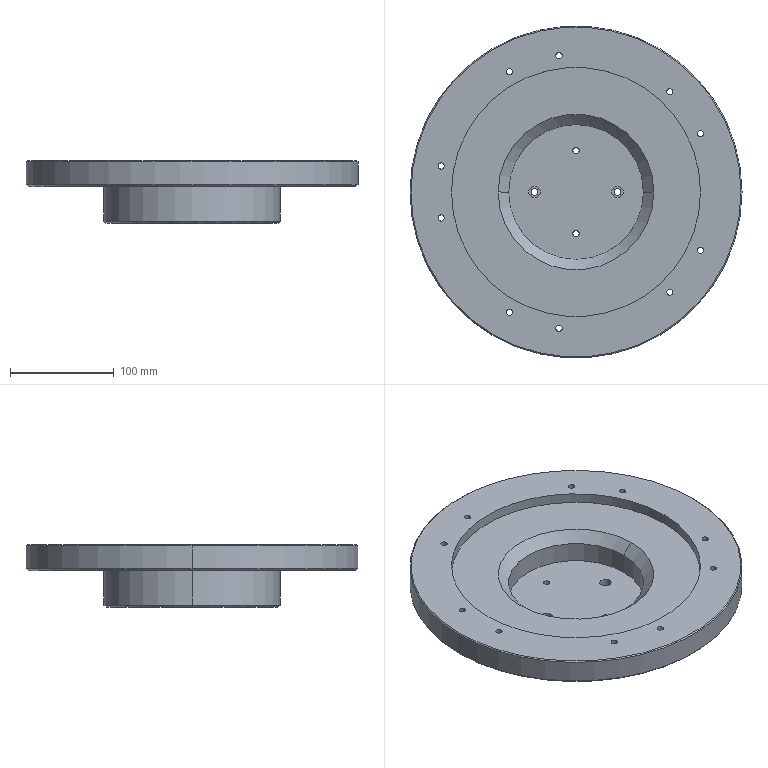NC program | NX | posted with a generic post | part box 320 x 320 x 60 mm
Lines 9378 to 10816 of 10816:
(DRILLING_COPY_1 , TOOL : D6A45)
N18742 T07 M6
N18744 G54
N18746 G17 G0 G90 X40. Y0. S3000 M3
N18748 G43 Z90. H7
N18750 G94 G81 G98 Z19. F200. R23.
N18752 X0. Y-40.
N18754 X-40. Y0.
N18756 X0. Y40.
N18758 Y0. Z59. R63.
N18760 X90.478 Y96.638
N18762 X119.867 Y56.187
N18764 Y-56.187
N18766 X90.478 Y-96.638
N18768 X-16.396 Y-131.363
N18770 X-63.949 Y-115.912
N18772 X-130. Y-25.
N18774 Y25.
N18776 X-63.949 Y115.912
N18778 X-16.396 Y131.363
N18780 G80
N18782 G0 X-16.396 Y131.363 Z90.
N18784 M5
(DRILLING_COPY_1_COPY_COPY_1 , TOOL : 5.8ZT)
N18786 T18 M6
N18788 G54
N18790 G17 G0 G90 X0. Y40. S2000 M3
N18792 G43 Z90. H18
N18794 G94 G83 G98 Z-3.242 F120. Q2. R23.
N18796 Y-40.
N18798 X-16.396 Y-131.363 Z31.758 R63.
N18800 X-63.949 Y-115.912
N18802 X-130. Y-25.
N18804 Y25.
N18806 X-63.949 Y115.912
N18808 X-16.396 Y131.363
N18810 X90.478 Y96.638
N18812 X119.867 Y56.187
N18814 Y-56.187
N18816 X90.478 Y-96.638
N18818 G80
N18820 G0 X90.478 Y-96.638 Z90.
N18822 M5
(DRILLING_COPY_1_COPY_COPY_1_COPY , TOOL : 6.0JD)
N18824 T19 M6
N18826 G54
N18828 G17 G0 G90 X0. Y40. S1000 M3
N18830 G43 Z90. H19
N18832 G94 G85 G98 Z-0.5 F40. R23.
N18834 Y-40.
N18836 X-16.396 Y-131.363 Z34.5 R63.
N18838 X-63.949 Y-115.912
N18840 X-130. Y-25.
N18842 Y25.
N18844 X-63.949 Y115.912
N18846 X-16.396 Y131.363
N18848 X90.478 Y96.638
N18850 X119.867 Y56.187
N18852 Y-56.187
N18854 X90.478 Y-96.638
N18856 G80
N18858 G0 X90.478 Y-96.638 Z90.
N18860 M5
(DRILLING_COPY_1_COPY_COPY_1_COPY_1 , TOOL : 6.6ZT)
N18862 T16 M6
N18864 G54
N18866 G17 G0 G90 X-40. Y0. S2000 M3
N18868 G43 Z90. H16
N18870 G94 G83 G98 Z-3.483 F120. Q2. R23.
N18872 X40.
N18874 G80
N18876 G0 X40. Y0. Z90.
N18878 M5
(HOLE_MILLING , TOOL : D6)
N18880 T06 M6
N18882 G54
N18884 G17 G0 G90 X-40. Y0. S7000 M3
N18886 G43 Z90. H6
N18888 Z20.5
N18890 G94 G3 X-38.75 Y-1.25 R1.25 F1000.
N18892 X-37.5 Y0. R1.25
N18894 X-37.5 Y0. Z20.2 I-2.5 J0.
N18896 X-37.5 Y0. Z19.9 I-2.5 J0.
N18898 X-37.5 Y0. Z19.6 I-2.5 J0.
N18900 X-37.5 Y0. Z19.3 I-2.5 J0.
N18902 X-37.5 Y0. Z19. I-2.5 J0.
N18904 X-37.5 Y0. Z18.7 I-2.5 J0.
N18906 X-37.5 Y0. Z18.4 I-2.5 J0.
N18908 X-37.5 Y0. Z18.1 I-2.5 J0.
N18910 X-37.5 Y0. Z17.8 I-2.5 J0.
N18912 X-37.5 Y0. Z17.5 I-2.5 J0.
N18914 X-37.5 Y0. Z17.2 I-2.5 J0.
N18916 X-37.5 Y0. Z16.9 I-2.5 J0.
N18918 X-37.5 Y0. Z16.6 I-2.5 J0.
N18920 X-37.5 Y0. Z16.3 I-2.5 J0.
N18922 X-37.5 Y0. Z16. I-2.5 J0.
N18924 X-37.5 Y0. Z15.7 I-2.5 J0.
N18926 X-37.5 Y0. Z15.4 I-2.5 J0.
N18928 X-37.5 Y0. Z15.1 I-2.5 J0.
N18930 X-37.5 Y0. Z14.8 I-2.5 J0.
N18932 X-37.5 Y0. Z14.5 I-2.5 J0.
N18934 X-37.5 Y0. Z14.2 I-2.5 J0.
N18936 X-37.5 Y0. Z13.9 I-2.5 J0.
N18938 X-37.5 Y0. Z13.6 I-2.5 J0.
N18940 X-37.5 Y0. Z13.3 I-2.5 J0.
N18942 X-41.25 Y2.165 Z13.2 R2.5
N18944 X-42.165 Y-1.25 R2.5
N18946 X-41.25 Y2.165 R-2.5
N18948 X-41.708 Y0.458 R1.25
N18950 X-40. Y0. R1.25
N18952 G0 Z90.
N18954 X40.
N18956 Z20.5
N18958 G3 X41.25 Y-1.25 R1.25
N18960 X42.5 Y0. R1.25
N18962 X42.5 Y0. Z20.2 I-2.5 J0.
N18964 X42.5 Y0. Z19.9 I-2.5 J0.
N18966 X42.5 Y0. Z19.6 I-2.5 J0.
N18968 X42.5 Y0. Z19.3 I-2.5 J0.
N18970 X42.5 Y0. Z19. I-2.5 J0.
N18972 X42.5 Y0. Z18.7 I-2.5 J0.
N18974 X42.5 Y0. Z18.4 I-2.5 J0.
N18976 X42.5 Y0. Z18.1 I-2.5 J0.
N18978 X42.5 Y0. Z17.8 I-2.5 J0.
N18980 X42.5 Y0. Z17.5 I-2.5 J0.
N18982 X42.5 Y0. Z17.2 I-2.5 J0.
N18984 X42.5 Y0. Z16.9 I-2.5 J0.
N18986 X42.5 Y0. Z16.6 I-2.5 J0.
N18988 X42.5 Y0. Z16.3 I-2.5 J0.
N18990 X42.5 Y0. Z16. I-2.5 J0.
N18992 X42.5 Y0. Z15.7 I-2.5 J0.
N18994 X42.5 Y0. Z15.4 I-2.5 J0.
N18996 X42.5 Y0. Z15.1 I-2.5 J0.
N18998 X42.5 Y0. Z14.8 I-2.5 J0.
N19000 X42.5 Y0. Z14.5 I-2.5 J0.
N19002 X42.5 Y0. Z14.2 I-2.5 J0.
N19004 X42.5 Y0. Z13.9 I-2.5 J0.
N19006 X42.5 Y0. Z13.6 I-2.5 J0.
N19008 X42.5 Y0. Z13.3 I-2.5 J0.
N19010 X38.75 Y2.165 Z13.2 R2.5
N19012 X37.835 Y-1.25 R2.5
N19014 X38.75 Y2.165 R-2.5
N19016 X38.292 Y0.458 R1.25
N19018 X40. Y0. R1.25
N19020 G0 Z90.
N19022 M5
(ZLEVEL_PROFILE_COPY_COPY_1_COPY_COPY_2_COPY_1 , TOOL : D6R0.5)
N19024 T05 M6
N19026 G54
N19028 G17 G0 G90 X-69.187 Y2.097 S7000 M3
N19030 G43 Z90. H5
N19032 Z49.929
N19034 G94 G1 X-71.919 Y0.52 F3000.
N19036 G3 X-72.219 Y0. R0.6
N19038 X0. Y-72.219 R72.219
N19040 X-72.219 Y0. R-72.219
N19042 G1 X-72.187 Z49.894
N19044 X-72.145 Z49.859
N19046 G2 X0.002 Y72.146 R72.147
N19048 X-72.145 Y0. R-72.147
N19050 G1 X-72.116 Z49.823
N19052 X-72.081 Z49.788
N19054 G3 X0. Y-72.081 R72.081
N19056 X-72.081 Y0. R-72.081
N19058 G1 X-72.01 Z49.717
N19060 G2 X0. Y72.01 R72.01
N19062 X-72.01 Y0. R-72.01
N19064 G1 X-71.939 Z49.646
N19066 G3 X0. Y-71.939 R71.939
N19068 X-71.939 Y0. R-71.939
N19070 G1 X-71.869 Z49.576
N19072 G2 X0. Y71.869 R71.869
N19074 X-71.869 Y0. R-71.869
N19076 G1 X-71.798 Z49.505
N19078 Y-0.003
N19080 G3 X0.003 Y-71.798 R71.798
N19082 X-71.798 Y0. R-71.798
N19084 G1 X-71.727 Z49.434
N19086 G2 X0. Y71.727 R71.727
N19088 X-71.727 Y0. R-71.727
N19090 G1 X-71.657 Z49.364
N19092 Y-0.003
N19094 G3 X0.003 Y-71.657 R71.657
N19096 X-71.657 Y0. R-71.657
N19098 G1 X-71.586 Z49.293
N19100 G2 X0. Y71.586 R71.586
N19102 X-71.586 Y0. R-71.586
N19104 G1 X-71.515 Z49.222
N19106 Y-0.003
N19108 G3 X0.003 Y-71.515 R71.515
N19110 X-71.515 Y0. R-71.515
N19112 G1 X-71.444 Z49.151
N19114 G2 X0. Y71.444 R71.444
N19116 X-71.444 Y0. R-71.444
N19118 G1 X-71.374 Z49.081
N19120 Y-0.005
N19122 G3 X0.005 Y-71.374 R71.374
N19124 X-71.374 Y0. R-71.374
N19126 G1 X-71.303 Z49.01
N19128 G2 X0. Y71.303 R71.303
N19130 X-71.303 Y0. R-71.303
N19132 G1 X-71.232 Z48.939
N19134 Y-0.005
N19136 G3 X0.005 Y-71.232 R71.232
N19138 X-71.232 Y0. R-71.232
N19140 G1 X-71.162 Z48.869
N19142 G2 X0. Y71.162 R71.162
N19144 X-71.162 Y0. R-71.162
N19146 G1 X-71.091 Z48.798
N19148 Y-0.003
N19150 G3 X0.003 Y-71.091 R71.091
N19152 X-71.091 Y0. R-71.091
N19154 G1 X-71.02 Z48.727
N19156 G2 X0. Y71.02 R71.02
N19158 X-71.02 Y0. R-71.02
N19160 G1 X-70.949 Z48.657
N19162 Y-0.003
N19164 G3 X0.003 Y-70.949 R70.949
N19166 X-70.949 Y0. R-70.949
N19168 G1 X-70.879 Z48.586
N19170 G2 X0. Y70.879 R70.879
N19172 X-70.879 Y0. R-70.879
N19174 G1 X-70.808 Z48.515
N19176 Y-0.003
N19178 G3 X0.003 Y-70.808 R70.808
N19180 X-70.808 Y0. R-70.808
N19182 G1 X-70.737 Z48.444
N19184 Y0.005
N19186 G2 X0.005 Y70.737 R70.737
N19188 X-70.737 Y0. R-70.737
N19190 G1 X-70.667 Z48.374
N19192 G3 X0. Y-70.667 R70.667
N19194 X-70.667 Y0. R-70.667
N19196 G1 X-70.596 Z48.303
N19198 Y0.005
N19200 G2 X0.005 Y70.596 R70.596
N19202 X-70.596 Y0. R-70.596
N19204 G1 X-70.525 Z48.232
N19206 G3 X0. Y-70.525 R70.525
N19208 X-70.525 Y0. R-70.525
N19210 G1 X-70.454 Z48.162
N19212 Y0.005
N19214 G2 X0.005 Y70.454 R70.454
N19216 X-70.454 Y0. R-70.454
N19218 G1 X-70.384 Z48.091
N19220 Y-0.003
N19222 G3 X0.003 Y-70.384 R70.384
N19224 X-70.384 Y0. R-70.384
N19226 G1 X-70.313 Z48.02
N19228 G2 X0. Y70.313 R70.313
N19230 X-70.313 Y0. R-70.313
N19232 G1 X-70.242 Z47.949
N19234 Y-0.003
N19236 G3 X0.003 Y-70.242 R70.242
N19238 X-70.242 Y0. R-70.242
N19240 G1 X-70.172 Z47.879
N19242 G2 X0. Y70.172 R70.172
N19244 X-70.172 Y0. R-70.172
N19246 G1 X-70.101 Z47.808
N19248 G3 X0. Y-70.101 R70.101
N19250 X-70.101 Y0. R-70.101
N19252 G1 X-70.03 Z47.737
N19254 Y0.005
N19256 G2 X0.005 Y70.03 R70.03
N19258 X-70.03 Y0. R-70.03
N19260 G1 X-69.959 Z47.667
N19262 G3 X0. Y-69.959 R69.959
N19264 X-69.959 Y0. R-69.959
N19266 G1 X-69.889 Z47.596
N19268 Y0.005
N19270 G2 X0.005 Y69.889 R69.889
N19272 X-69.889 Y0. R-69.889
N19274 G1 X-69.818 Z47.525
N19276 G3 X0. Y-69.818 R69.818
N19278 X-69.818 Y0. R-69.818
N19280 G1 X-69.747 Z47.454
N19282 G2 X0. Y69.747 R69.747
N19284 X-69.747 Y0. R-69.747
N19286 G1 X-69.677 Z47.384
N19288 Y-0.003
N19290 G3 X0.003 Y-69.677 R69.677
N19292 X-69.677 Y0. R-69.677
N19294 G1 X-69.606 Z47.313
N19296 G2 X0. Y69.606 R69.606
N19298 X-69.606 Y0. R-69.606
N19300 G1 X-69.535 Z47.242
N19302 Y-0.003
N19304 G3 X0.003 Y-69.535 R69.535
N19306 X-69.535 Y0. R-69.535
N19308 G1 X-69.464 Z47.172
N19310 G2 X0. Y69.464 R69.464
N19312 X-69.464 Y0. R-69.464
N19314 G1 X-69.394 Z47.101
N19316 G3 X0. Y-69.394 R69.394
N19318 X-69.394 Y0. R-69.394
N19320 G1 X-69.323 Z47.03
N19322 Y0.005
N19324 G2 X0.005 Y69.323 R69.323
N19326 X-69.323 Y0. R-69.323
N19328 G1 X-69.252 Z46.959
N19330 G3 X0. Y-69.252 R69.252
N19332 X-69.252 Y0. R-69.252
N19334 G1 X-69.182 Z46.889
N19336 Y0.005
N19338 G2 X0.005 Y69.182 R69.182
N19340 X-69.182 Y0. R-69.182
N19342 G1 X-69.111 Z46.818
N19344 G3 X0. Y-69.111 R69.111
N19346 X-69.111 Y0. R-69.111
N19348 G1 X-69.04 Z46.747
N19350 G2 X0. Y69.04 R69.04
N19352 X-69.04 Y0. R-69.04
N19354 G1 X-68.97 Z46.677
N19356 Y-0.003
N19358 G3 X0.003 Y-68.97 R68.97
N19360 X-68.97 Y0. R-68.97
N19362 G1 X-68.899 Z46.606
N19364 G2 X0. Y68.899 R68.899
N19366 X-68.899 Y0. R-68.899
N19368 G1 X-68.828 Z46.535
N19370 Y-0.003
N19372 G3 X0.003 Y-68.828 R68.828
N19374 X-68.828 Y0. R-68.828
N19376 G1 X-68.757 Z46.464
N19378 G2 X0. Y68.757 R68.757
N19380 X-68.757 Y0. R-68.757
N19382 G1 X-68.687 Z46.394
N19384 G3 X0. Y-68.687 R68.687
N19386 X-68.687 Y0. R-68.687
N19388 G1 X-68.616 Z46.323
N19390 Y0.005
N19392 G2 X0.005 Y68.616 R68.616
N19394 X-68.616 Y0. R-68.616
N19396 G1 X-68.545 Z46.252
N19398 G3 X0. Y-68.545 R68.545
N19400 X-68.545 Y0. R-68.545
N19402 G1 X-68.475 Z46.182
N19404 Y0.005
N19406 G2 X0.005 Y68.475 R68.475
N19408 X-68.475 Y0. R-68.475
N19410 G1 X-68.404 Z46.111
N19412 G3 X0. Y-68.404 R68.404
N19414 X-68.404 Y0. R-68.404
N19416 G1 X-68.333 Z46.04
N19418 G2 X0. Y68.333 R68.333
N19420 X-68.333 Y0. R-68.333
N19422 G1 X-68.262 Z45.97
N19424 Y-0.003
N19426 G3 X0.003 Y-68.262 R68.262
N19428 X-68.262 Y0. R-68.262
N19430 G1 X-68.192 Z45.899
N19432 G2 X0. Y68.192 R68.192
N19434 X-68.192 Y0. R-68.192
N19436 G1 X-68.121 Z45.828
N19438 Y-0.003
N19440 G3 X0.003 Y-68.121 R68.121
N19442 X-68.121 Y0. R-68.121
N19444 G1 X-68.05 Z45.757
N19446 G2 X0. Y68.05 R68.05
N19448 X-68.05 Y0. R-68.05
N19450 G1 X-67.98 Z45.687
N19452 G3 X0. Y-67.98 R67.98
N19454 X-67.98 Y0. R-67.98
N19456 G1 X-67.909 Z45.616
N19458 Y0.005
N19460 G2 X0.005 Y67.909 R67.909
N19462 X-67.909 Y0. R-67.909
N19464 G1 X-67.838 Z45.545
N19466 G3 X0. Y-67.838 R67.838
N19468 X-67.838 Y0. R-67.838
N19470 G1 X-67.767 Z45.475
N19472 Y0.005
N19474 G2 X0.005 Y67.767 R67.767
N19476 X-67.767 Y0. R-67.767
N19478 G1 X-67.697 Z45.404
N19480 G3 X0. Y-67.697 R67.697
N19482 X-67.697 Y0. R-67.697
N19484 G1 X-67.626 Z45.333
N19486 G2 X0. Y67.626 R67.626
N19488 X-67.626 Y0. R-67.626
N19490 G1 X-67.555 Z45.262
N19492 Y-0.003
N19494 G3 X0.003 Y-67.555 R67.555
N19496 X-67.555 Y0. R-67.555
N19498 G1 X-67.485 Z45.192
N19500 G2 X0. Y67.485 R67.485
N19502 X-67.485 Y0. R-67.485
N19504 G1 X-67.414 Z45.121
N19506 Y-0.003
N19508 G3 X0.003 Y-67.414 R67.414
N19510 X-67.414 Y0. R-67.414
N19512 G1 X-67.343 Z45.05
N19514 G2 X0. Y67.343 R67.343
N19516 X-67.343 Y0. R-67.343
N19518 G1 X-67.272 Z44.98
N19520 G3 X0. Y-67.272 R67.272
N19522 X-67.272 Y0. R-67.272
N19524 G1 X-67.202 Z44.909
N19526 Y0.005
N19528 G2 X0.005 Y67.202 R67.202
N19530 X-67.202 Y0. R-67.202
N19532 G1 X-67.131 Z44.838
N19534 G3 X0. Y-67.131 R67.131
N19536 X-67.131 Y0. R-67.131
N19538 G1 X-67.06 Z44.767
N19540 Y0.005
N19542 G2 X0.005 Y67.06 R67.06
N19544 X-67.06 Y0. R-67.06
N19546 G1 X-66.99 Z44.697
N19548 Y-0.003
N19550 G3 X0.003 Y-66.99 R66.99
N19552 X-66.99 Y0. R-66.99
N19554 G1 X-66.919 Z44.626
N19556 G2 X0. Y66.919 R66.919
N19558 X-66.919 Y0. R-66.919
N19560 G1 X-66.848 Z44.555
N19562 Y-0.003
N19564 G3 X0.003 Y-66.848 R66.848
N19566 X-66.848 Y0. R-66.848
N19568 G1 X-66.777 Z44.485
N19570 G2 X0. Y66.777 R66.777
N19572 X-66.777 Y0. R-66.777
N19574 G1 X-66.707 Z44.414
N19576 Y-0.003
N19578 G3 X0.003 Y-66.707 R66.707
N19580 X-66.707 Y0. R-66.707
N19582 G1 X-66.636 Z44.343
N19584 G2 X0. Y66.636 R66.636
N19586 X-66.636 Y0. R-66.636
N19588 G1 X-66.565 Z44.272
N19590 Y-0.005
N19592 G3 X0.005 Y-66.565 R66.565
N19594 X-66.565 Y0. R-66.565
N19596 G1 X-66.495 Z44.202
N19598 G2 X0. Y66.495 R66.495
N19600 X-66.495 Y0. R-66.495
N19602 G1 X-66.424 Z44.131
N19604 Y-0.005
N19606 G3 X0.005 Y-66.424 R66.424
N19608 X-66.424 Y0. R-66.424
N19610 G1 X-66.353 Z44.06
N19612 G2 X0. Y66.353 R66.353
N19614 X-66.353 Y0. R-66.353
N19616 G1 X-66.282 Z43.99
N19618 Y-0.003
N19620 G3 X0.003 Y-66.282 R66.282
N19622 X-66.282 Y0. R-66.282
N19624 G1 X-66.212 Z43.919
N19626 G2 X0. Y66.212 R66.212
N19628 X-66.212 Y0. R-66.212
N19630 G1 X-66.141 Z43.848
N19632 Y-0.003
N19634 G3 X0.003 Y-66.141 R66.141
N19636 X-66.141 Y0. R-66.141
N19638 G1 X-66.07 Z43.777
N19640 G2 X0. Y66.07 R66.07
N19642 X-66.07 Y0. R-66.07
N19644 G1 X-66. Z43.707
N19646 Y-0.003
N19648 G3 X0.003 Y-66. R66.
N19650 X-66. Y0. R-66.
N19652 G1 X-65.929 Z43.636
N19654 G2 X0. Y65.929 R65.929
N19656 X-65.929 Y0. R-65.929
N19658 G1 X-65.858 Z43.565
N19660 Y-0.005
N19662 G3 X0.005 Y-65.858 R65.858
N19664 X-65.858 Y0. R-65.858
N19666 G1 X-65.788 Z43.495
N19668 G2 X0. Y65.788 R65.788
N19670 X-65.788 Y0. R-65.788
N19672 G1 X-65.717 Z43.424
N19674 Y-0.005
N19676 G3 X0.005 Y-65.717 R65.717
N19678 X-65.717 Y0. R-65.717
N19680 G1 X-65.646 Z43.353
N19682 G2 X0. Y65.646 R65.646
N19684 X-65.646 Y0. R-65.646
N19686 G1 X-65.575 Z43.282
N19688 Y-0.003
N19690 G3 X0.003 Y-65.575 R65.575
N19692 X-65.575 Y0. R-65.575
N19694 G1 X-65.505 Z43.212
N19696 G2 X0. Y65.505 R65.505
N19698 X-65.505 Y0. R-65.505
N19700 G1 X-65.434 Z43.141
N19702 Y-0.003
N19704 G3 X0.003 Y-65.434 R65.434
N19706 X-65.434 Y0. R-65.434
N19708 G1 X-65.363 Z43.07
N19710 G2 X0. Y65.363 R65.363
N19712 X-65.363 Y0. R-65.363
N19714 G1 X-65.293 Z43.
N19716 Y-0.003
N19718 G3 X0.003 Y-65.293 R65.293
N19720 X-65.293 Y0. R-65.293
N19722 G1 X-65.222 Z42.929
N19724 G2 X0. Y65.222 R65.222
N19726 X-65.222 Y0. R-65.222
N19728 G1 X-65.151 Z42.858
N19730 Y-0.005
N19732 G3 X0.005 Y-65.151 R65.151
N19734 X-65.151 Y0. R-65.151
N19736 G1 X-65.08 Z42.788
N19738 G2 X0. Y65.08 R65.08
N19740 X-65.08 Y0. R-65.08
N19742 G1 X-65.01 Z42.717
N19744 Y-0.005
N19746 G3 X0.005 Y-65.01 R65.01
N19748 X-65.01 Y0. R-65.01
N19750 G1 X-64.939 Z42.646
N19752 G2 X0. Y64.939 R64.939
N19754 X-64.939 Y0. R-64.939
N19756 G1 X-64.868 Z42.575
N19758 Y-0.003
N19760 G3 X0.003 Y-64.868 R64.868
N19762 X-64.868 Y0. R-64.868
N19764 G1 X-64.798 Z42.505
N19766 G2 X0. Y64.798 R64.798
N19768 X-64.798 Y0. R-64.798
N19770 G1 X-64.727 Z42.434
N19772 Y-0.003
N19774 G3 X0.003 Y-64.727 R64.727
N19776 X-64.727 Y0. R-64.727
N19778 G1 X-64.656 Z42.363
N19780 G2 X0. Y64.656 R64.656
N19782 X-64.656 Y0. R-64.656
N19784 G1 X-64.585 Z42.293
N19786 Y-0.003
N19788 G3 X0.003 Y-64.585 R64.585
N19790 X-64.585 Y0. R-64.585
N19792 G1 X-64.515 Z42.222
N19794 G2 X0. Y64.515 R64.515
N19796 X-64.515 Y0. R-64.515
N19798 G1 X-64.444 Z42.151
N19800 Y-0.005
N19802 G3 X0.005 Y-64.444 R64.444
N19804 X-64.444 Y0. R-64.444
N19806 G1 X-64.373 Z42.08
N19808 G2 X0. Y64.373 R64.373
N19810 X-64.373 Y0. R-64.373
N19812 G1 X-64.303 Z42.01
N19814 Y-0.005
N19816 G3 X0.005 Y-64.303 R64.303
N19818 X-64.303 Y0. R-64.303
N19820 G1 X-64.232 Z41.939
N19822 G2 X0. Y64.232 R64.232
N19824 X-64.232 Y0. R-64.232
N19826 G1 X-64.161 Z41.868
N19828 Y-0.003
N19830 G3 X0.003 Y-64.161 R64.161
N19832 X-64.161 Y0. R-64.161
N19834 G1 X-64.09 Z41.798
N19836 G2 X0. Y64.09 R64.09
N19838 X-64.09 Y0. R-64.09
N19840 G1 X-64.02 Z41.727
N19842 Y-0.003
N19844 G3 X0.003 Y-64.02 R64.02
N19846 X-64.02 Y0. R-64.02
N19848 G1 X-63.949 Z41.656
N19850 G2 X0. Y63.949 R63.949
N19852 X-63.949 Y0. R-63.949
N19854 G1 X-63.878 Z41.585
N19856 Y-0.003
N19858 G3 X0.003 Y-63.878 R63.878
N19860 X-63.878 Y0. R-63.878
N19862 G1 X-63.808 Z41.515
N19864 G2 X0. Y63.808 R63.808
N19866 X-63.808 Y0. R-63.808
N19868 G1 X-63.737 Z41.444
N19870 Y-0.005
N19872 G3 X0.005 Y-63.737 R63.737
N19874 X-63.737 Y0. R-63.737
N19876 G1 X-63.666 Z41.373
N19878 G2 X0. Y63.666 R63.666
N19880 X-63.666 Y0. R-63.666
N19882 G1 X-63.595 Z41.303
N19884 Y-0.005
N19886 G3 X0.005 Y-63.595 R63.595
N19888 X-63.595 Y0. R-63.595
N19890 G1 X-63.525 Z41.232
N19892 G2 X0. Y63.525 R63.525
N19894 X-63.525 Y0. R-63.525
N19896 G1 X-63.454 Z41.161
N19898 Y-0.003
N19900 G3 X0.003 Y-63.454 R63.454
N19902 X-63.454 Y0. R-63.454
N19904 G1 X-63.383 Z41.09
N19906 G2 X0. Y63.383 R63.383
N19908 X-63.383 Y0. R-63.383
N19910 G1 X-63.313 Z41.02
N19912 Y-0.003
N19914 G3 X0.003 Y-63.313 R63.313
N19916 X-63.313 Y0. R-63.313
N19918 G1 X-63.242 Z40.949
N19920 G2 X0. Y63.242 R63.242
N19922 X-63.242 Y0. R-63.242
N19924 G1 X-63.171 Z40.878
N19926 G3 X0. Y-63.171 R63.171
N19928 X-63.171 Y0. R-63.171
N19930 G1 X-63.101 Z40.808
N19932 Y0.005
N19934 G2 X0.005 Y63.101 R63.101
N19936 X-63.101 Y0. R-63.101
N19938 G1 X-63.03 Z40.737
N19940 G3 X0. Y-63.03 R63.03
N19942 X-63.03 Y0. R-63.03
N19944 G1 X-62.959 Z40.666
N19946 Y0.005
N19948 G2 X0.005 Y62.959 R62.959
N19950 X-62.959 Y0. R-62.959
N19952 G1 X-62.888 Z40.595
N19954 G3 X0. Y-62.888 R62.888
N19956 X-62.888 Y0. R-62.888
N19958 G1 X-62.818 Z40.525
N19960 G2 X0. Y62.818 R62.818
N19962 X-62.818 Y0. R-62.818
N19964 G1 X-62.747 Z40.454
N19966 Y-0.003
N19968 G3 X0.003 Y-62.747 R62.747
N19970 X-62.747 Y0. R-62.747
N19972 G1 X-62.676 Z40.383
N19974 G2 X0. Y62.676 R62.676
N19976 X-62.676 Y0. R-62.676
N19978 G1 X-62.606 Z40.313
N19980 Y-0.003
N19982 G3 X0.003 Y-62.606 R62.606
N19984 X-62.606 Y0. R-62.606
N19986 G1 X-62.535 Z40.242
N19988 G2 X0. Y62.535 R62.535
N19990 X-62.535 Y0. R-62.535
N19992 G1 X-62.464 Z40.171
N19994 G3 X0. Y-62.464 R62.464
N19996 X-62.464 Y0. R-62.464
N19998 G1 X-62.393 Z40.101
N20000 G2 X0. Y62.393 R62.393
N20002 X-62.393 Y0. R-62.393
N20004 G1 X-62.323 Z40.03
N20006 G3 X0. Y-62.323 R62.323
N20008 X-62.323 Y0. R-62.323
N20010 G1 X-62.252 Z39.959
N20012 G2 X0. Y62.252 R62.252
N20014 X-62.252 Y0. R-62.252
N20016 G1 X-62.181 Z39.888
N20018 G3 X0. Y-62.181 R62.181
N20020 X-62.181 Y0. R-62.181
N20022 G1 X-62.146 Z39.853
N20024 X-62.109 Z39.818
N20026 G2 X-0.001 Y62.11 R62.109
N20028 X-62.109 Y0. R-62.109
N20030 G1 X-62.075 Z39.782
N20032 X-62.038 Z39.747
N20034 G3 X0. Y-62.038 R62.038
N20036 X-62.038 Y0. R-62.038
N20038 G1 X-62.008 Z39.716
N20040 X-61.977 Z39.685
N20042 G2 X0. Y61.977 R61.977
N20044 X-61.977 Y0. R-61.977
N20046 G1 X-61.946 Z39.654
N20048 X-61.915 Z39.623
N20050 G3 X0. Y-61.915 R61.915
N20052 X-61.915 Y0. R-61.915
N20054 G1 X-61.884 Z39.593
N20056 X-61.852 Z39.562
N20058 G2 X0.001 Y61.851 R61.852
N20060 X-61.852 Y0. R-61.852
N20062 G1 X-61.822 Z39.531
N20064 X-61.79 Z39.5
N20066 G3 X0. Y-61.791 R61.79
N20068 X-61.79 Y0. R-61.79
N20070 X-61.49 Y-0.52 R0.6
N20072 G1 X-58.753 Y-2.1
N20074 G0 Z90.
N20076 M5
(FLOOR_WALL_1_COPY_1 , TOOL : D10JING)
N20078 T11 M6
N20080 G54
N20082 G17 G0 G90 X0.802 Y113.9 S7000 M3
N20084 G43 Z90. H11
N20086 Z51.5
N20088 G94 G1 Z50. F1000.
N20090 G3 X-0.064 Y114.4 R1.
N20092 G1 X0.061
N20094 G2 X33.365 Y109.427 R114.4
N20096 G1 X-33.368 Y109.426
N20098 G3 X-46.661 Y104.452 R114.4
N20100 G1 X46.658 Y104.453
N20102 G2 X56.492 Y99.479 R114.4
N20104 G1 X-56.494 Y99.478
N20106 G3 X-64.471 Y94.503 R114.4
N20108 G1 X64.468 Y94.505
N20110 G2 X71.214 Y89.531 R114.4
N20112 G1 X-71.217 Y89.529
N20114 G3 X-77.057 Y84.555 R114.4
N20116 G1 X77.054 Y84.558
N20118 G2 X82.181 Y79.584 R114.4
N20120 G1 X-82.184 Y79.582
N20122 G3 X-86.724 Y74.608 R114.4
N20124 G1 X86.722 Y74.61
N20126 G2 X90.764 Y69.636 R114.4
N20128 G1 X7.14 Y69.635
N20130 X26.813 Y64.661
N20132 X94.373 Y64.662
N20134 G2 X97.594 Y59.688 R114.4
N20136 G1 X36.571 Y59.687
N20138 X43.663 Y54.714
N20140 X100.467
N20142 G2 X103.021 Y49.74 R114.4
N20144 G1 X49.254
N20146 X53.815 Y44.766
N20148 X105.277 Y44.767
N20150 G2 X107.256 Y39.793 R114.4
N20152 G1 X57.59 Y39.792
N20154 X60.726 Y34.818
N20156 X108.973 Y34.819
N20158 G2 X110.438 Y29.845 R114.4
N20160 G1 X63.319 Y29.844
N20162 X65.433 Y24.87
N20164 X111.664 Y24.871
N20166 G2 X112.656 Y19.897 R114.4
N20168 G1 X67.113
N20170 X68.391 Y14.923
N20172 X113.422
N20174 G2 X113.967 Y9.949 R114.4
N20176 G1 X69.289
N20178 X69.823 Y4.975
N20180 X114.292
N20182 G2 X114.4 Y0.002 R114.4
N20184 G1 X70. Y0.001
N20186 X69.823 Y-4.973
N20188 X114.292 Y-4.972
N20190 G2 X113.967 Y-9.946 R114.4
N20192 G1 X69.29 Y-9.947
N20194 X68.391 Y-14.921
N20196 X113.423 Y-14.92
N20198 G2 X112.657 Y-19.894 R114.4
N20200 G1 X67.113 Y-19.895
N20202 X65.434 Y-24.869
N20204 X111.664 Y-24.868
N20206 G2 X110.439 Y-29.842 R114.4
N20208 G1 X63.32 Y-29.843
N20210 X60.727 Y-34.817
N20212 X108.973 Y-34.816
N20214 G2 X107.257 Y-39.79 R114.4
N20216 G1 X57.591 Y-39.791
N20218 X53.816 Y-44.765
N20220 X105.278 Y-44.764
N20222 G2 X103.022 Y-49.738 R114.4
N20224 G1 X49.255
N20226 X43.664 Y-54.712
N20228 X100.469
N20230 G2 X97.596 Y-59.686 R114.4
N20232 G1 X36.572
N20234 X26.815 Y-64.661
N20236 X94.374 Y-64.66
N20238 G2 X90.766 Y-69.634 R114.4
N20240 G1 X7.142 Y-69.635
N20242 G2 X6.276 Y-69.135 R1.
N20244 G1 Z51.5
N20246 G0 Z53.1
N20248 G1 X-7.96 Y69.06 F6000.
N20250 G0 Z51.5
N20252 G1 Z50. F1000.
N20254 G2 X-7.142 Y69.635 R1.
N20256 G1 X-90.766 Y69.634
N20258 G3 X-94.374 Y64.66 R114.4
N20260 G1 X-26.815 Y64.661
N20262 X-36.572 Y59.686
N20264 X-97.596
N20266 G3 X-100.469 Y54.712 R114.4
N20268 G1 X-43.664
N20270 X-49.255 Y49.738
N20272 X-103.022
N20274 G3 X-105.278 Y44.764 R114.4
N20276 G1 X-53.816 Y44.765
N20278 X-57.591 Y39.791
N20280 X-107.257 Y39.79
N20282 G3 X-108.973 Y34.816 R114.4
N20284 G1 X-60.727 Y34.817
N20286 X-63.32 Y29.843
N20288 X-110.439 Y29.842
N20290 G3 X-111.664 Y24.868 R114.4
N20292 G1 X-65.434 Y24.869
N20294 X-67.113 Y19.895
N20296 X-112.657 Y19.894
N20298 G3 X-113.423 Y14.92 R114.4
N20300 G1 X-68.391 Y14.921
N20302 X-69.29 Y9.947
N20304 X-113.967 Y9.946
N20306 G3 X-114.292 Y4.972 R114.4
N20308 G1 X-69.823 Y4.973
N20310 X-70. Y-0.001
N20312 X-114.4 Y-0.002
N20314 G3 X-114.292 Y-4.975 R114.4
N20316 G1 X-69.823
N20318 X-69.289 Y-9.949
N20320 X-113.967
N20322 G3 X-113.422 Y-14.923 R114.4
N20324 G1 X-68.391
N20326 X-67.113 Y-19.897
N20328 X-112.656
N20330 G3 X-111.664 Y-24.871 R114.4
N20332 G1 X-65.433 Y-24.87
N20334 X-63.319 Y-29.844
N20336 X-110.438 Y-29.845
N20338 G3 X-108.973 Y-34.819 R114.4
N20340 G1 X-60.726 Y-34.818
N20342 X-57.59 Y-39.792
N20344 X-107.256 Y-39.793
N20346 G3 X-105.277 Y-44.767 R114.4
N20348 G1 X-53.815 Y-44.766
N20350 X-49.254 Y-49.74
N20352 X-103.021
N20354 G3 X-100.467 Y-54.714 R114.4
N20356 G1 X-43.663
N20358 X-36.571 Y-59.687
N20360 X-97.594 Y-59.688
N20362 G3 X-94.373 Y-64.662 R114.4
N20364 G1 X-26.813 Y-64.661
N20366 X-7.14 Y-69.635
N20368 X-90.764 Y-69.636
N20370 G3 X-86.722 Y-74.61 R114.4
N20372 G1 X86.724 Y-74.608
N20374 G2 X82.184 Y-79.582 R114.4
N20376 G1 X-82.181 Y-79.584
N20378 G3 X-77.054 Y-84.558 R114.4
N20380 G1 X77.057 Y-84.555
N20382 G2 X71.217 Y-89.529 R114.4
N20384 G1 X-71.214 Y-89.531
N20386 G3 X-64.468 Y-94.505 R114.4
N20388 G1 X64.471 Y-94.503
N20390 G2 X56.494 Y-99.478 R114.4
N20392 G1 X-56.492 Y-99.479
N20394 G3 X-46.658 Y-104.453 R114.4
N20396 G1 X46.661 Y-104.452
N20398 G2 X33.368 Y-109.426 R114.4
N20400 G1 X-33.365 Y-109.427
N20402 G3 X-0.061 Y-114.4 R114.4
N20404 G1 X0.064
N20406 G3 X0.93 Y-113.9 R1.
N20408 G1 X-0.802 Y-114.4
N20410 G3 X0.064 Y-114.9 R1.
N20412 X114.9 Y0.064 R114.9
N20414 X0.064 Y-114.9 R-114.9
N20416 X0.93 Y-114.399 R1.
N20418 G1 X1.512 Y-113.39
N20420 Z51.5
N20422 G0 Z90.
N20424 X0.832 Y58.9
N20426 Z21.5
N20428 G1 Z20.
N20430 G3 X-0.034 Y59.4 R1.
N20432 G1 X0.032
N20434 G2 X23.738 Y54.45 R59.4
N20436 G1 X-23.74
N20438 G3 X-32.836 Y49.499 R59.4
N20440 G1 X32.834 Y49.501
N20442 G2 X39.289 Y44.551 R59.4
N20444 G1 X-39.29 Y44.549
N20446 G3 X-44.275 Y39.599 R59.4
N20448 G1 X44.273 Y39.601
N20450 G2 X48.246 Y34.651 R59.4
N20452 G1 X-48.247 Y34.649
N20454 G3 X-51.442 Y29.699 R59.4
N20456 G1 X51.441 Y29.701
N20458 G2 X53.998 Y24.751 R59.4
N20460 G1 X-53.999 Y24.749
N20462 G3 X-56.003 Y19.799 R59.4
N20464 G1 X56.002 Y19.801
N20466 G2 X57.514 Y14.851 R59.4
N20468 G1 X-57.514 Y14.849
N20470 G3 X-58.569 Y9.899 R59.4
N20472 G1 X58.569 Y9.901
N20474 G2 X59.193 Y4.951 R59.4
N20476 G1 X-59.193 Y4.949
N20478 G3 X-59.4 Y-0.001 R59.4
N20480 G1 X-40.5
N20482 X-39.5
N20484 X39.5 Y0.001
N20486 X40.5
N20488 X59.4
N20490 Y0.
N20492 G2 X59.193 Y-4.949 R59.4
N20494 G1 X-59.193 Y-4.951
N20496 G3 X-58.569 Y-9.901 R59.4
N20498 G1 X58.569 Y-9.899
N20500 G2 X57.514 Y-14.849 R59.4
N20502 G1 X-57.514 Y-14.851
N20504 G3 X-56.002 Y-19.801 R59.4
N20506 G1 X56.003 Y-19.799
N20508 G2 X53.999 Y-24.749 R59.4
N20510 G1 X-53.998 Y-24.751
N20512 G3 X-51.441 Y-29.701 R59.4
N20514 G1 X51.442 Y-29.699
N20516 G2 X48.247 Y-34.649 R59.4
N20518 G1 X-48.246 Y-34.651
N20520 G3 X-44.273 Y-39.601 R59.4
N20522 G1 X44.275 Y-39.599
N20524 G2 X39.29 Y-44.549 R59.4
N20526 G1 X-39.289 Y-44.551
N20528 G3 X-32.834 Y-49.501 R59.4
N20530 G1 X32.836 Y-49.499
N20532 G2 X23.74 Y-54.45 R59.4
N20534 G1 X-23.738
N20536 G3 X-0.032 Y-59.4 R59.4
N20538 G1 X0.034
N20540 G3 X0.9 Y-58.9 R1.
N20542 G1 X-0.832 Y-59.4
N20544 G3 X0.034 Y-59.9 R1.
N20546 X59.9 Y0.034 R59.9
N20548 X0.034 Y-59.9 R-59.9
N20550 X0.9 Y-59.399 R1.
N20552 G1 X1.487 Y-58.381
N20554 Z21.5
N20556 G0 Z90.
N20558 M5
(ZLEVEL_PROFILE_COPY_1_COPY_COPY_COPY_COPY_2_COPY , TOOL : D6A45)
N20560 T07 M6
N20562 G54
N20564 G17 G0 G90 X-130.806 Y25.241 S7000 M3
N20566 G43 Z90. H7
N20568 Z59.
N20570 G94 G1 X-131.741 Y25.52 F1000.
N20572 G3 X-132.041 Y25. R0.6
N20574 X-130. Y22.959 R2.041
N20576 X-132.041 Y25. R-2.041
N20578 X-131.741 Y24.48 R0.6
N20580 G1 X-130.806 Y24.759
N20582 G0 Z90.
N20584 Y-24.759
N20586 Z59.
N20588 G1 X-131.741 Y-24.48
N20590 G3 X-132.041 Y-25. R0.6
N20592 G1 Y-25.001
N20594 G3 X-129.999 Y-27.041 R2.041
N20596 X-132.041 Y-25. R-2.041
N20598 X-131.741 Y-25.52 R0.6
N20600 G1 X-130.806 Y-25.241
N20602 G0 Z90.
N20604 X-16.155 Y132.169
N20606 Z59.
N20608 G1 X-15.876 Y133.104
N20610 G3 X-16.396 Y133.404 R0.6
N20612 X-18.437 Y131.363 R2.041
N20614 X-16.396 Y133.404 R-2.041
N20616 X-16.915 Y133.104 R0.6
N20618 G1 X-16.636 Y132.169
N20620 G0 Z90.
N20622 X90.237 Y-97.444
N20624 Z59.
N20626 G1 X89.958 Y-98.379
N20628 G3 X90.478 Y-98.679 R0.6
N20630 X92.519 Y-96.638 R2.041
N20632 X90.478 Y-98.679 R-2.041
N20634 X90.997 Y-98.379 R0.6
N20636 G1 X90.718 Y-97.444
N20638 G0 Z90.
N20640 X-64.189 Y-116.718
N20642 Z59.
N20644 G1 X-64.468 Y-117.653
N20646 G3 X-63.949 Y-117.953 R0.6
N20648 X-61.907 Y-115.912 R2.041
N20650 X-63.949 Y-117.953 R-2.041
N20652 X-63.429 Y-117.653 R0.6
N20654 G1 X-63.708 Y-116.718
N20656 G0 Z90.
N20658 X120.673 Y55.946
N20660 Z59.
N20662 G1 X121.608 Y55.667
N20664 G3 X121.908 Y56.187 R0.6
N20666 G1 Y56.189
N20668 G3 X119.864 Y58.228 R2.041
N20670 X121.908 Y56.187 R-2.041
N20672 X121.608 Y56.706 R0.6
N20674 G1 X120.673 Y56.427
N20676 G0 Z90.
N20678 Y-56.427
N20680 Z59.
N20682 G1 X121.608 Y-56.706
N20684 G3 X121.908 Y-56.187 R0.6
N20686 X119.867 Y-54.145 R2.041
N20688 X121.908 Y-56.187 R-2.041
N20690 X121.608 Y-55.667 R0.6
N20692 G1 X120.673 Y-55.946
N20694 G0 Z90.
N20696 X117.837 Y-1.042
N20698 Z59.
N20700 G1 X118.741 Y-0.52
N20702 G3 X119.041 Y0. R0.6
N20704 X0. Y119.041 R119.041
N20706 X119.041 Y0. R-119.041
N20708 X118.741 Y0.52 R0.6
N20710 G1 X117.837 Y1.042
N20712 G0 Z90.
N20714 X-16.636 Y-132.169
N20716 Z59.
N20718 G1 X-16.915 Y-133.104
N20720 G3 X-16.396 Y-133.404 R0.6
N20722 X-14.354 Y-131.363 R2.041
N20724 X-16.396 Y-133.404 R-2.041
N20726 X-15.876 Y-133.104 R0.6
N20728 G1 X-16.155 Y-132.169
N20730 G0 Z90.
N20732 X90.718 Y97.444
N20734 Z59.
N20736 G1 X90.997 Y98.379
N20738 G3 X90.478 Y98.679 R0.6
N20740 X88.436 Y96.638 R2.041
N20742 X90.478 Y98.679 R-2.041
N20744 X89.958 Y98.379 R0.6
N20746 G1 X90.237 Y97.444
N20748 G0 Z90.
N20750 X-63.708 Y116.718
N20752 Z59.
N20754 G1 X-63.429 Y117.653
N20756 G3 X-63.949 Y117.953 R0.6
N20758 X-65.99 Y115.912 R2.041
N20760 X-63.949 Y117.953 R-2.041
N20762 X-64.468 Y117.653 R0.6
N20764 G1 X-64.189 Y116.718
N20766 G0 Z90.
N20768 X-1.037 Y161.126
N20770 Z59.
N20772 G1 X-0.52 Y160.229
N20774 G3 X0. Y159.929 R0.6
N20776 G2 X159.929 Y0. R159.929
N20778 X0. Y159.929 R-159.929
N20780 G3 X0.52 Y160.229 R0.6
N20782 G1 X1.037 Y161.126
N20784 G0 Z90.
(ZLEVEL_PROFILE_COPY_1_COPY_COPY_COPY_COPY_2_COPY_COPY , TOOL : D6A45)
N20786 X43.134 Y-1.159
N20788 Z19.
N20790 G1 X44.241 Y-0.52
N20792 G3 X44.541 Y0. R0.6
N20794 X40. Y4.541 R4.541
N20796 X44.541 Y0. R-4.541
N20798 X44.241 Y0.52 R0.6
N20800 G1 X43.134 Y1.159
N20802 G0 Z90.
N20804 X-0.241 Y-40.806
N20806 Z19.
N20808 G1 X-0.52 Y-41.741
N20810 G3 X0. Y-42.041 R0.6
N20812 X2.041 Y-40. R2.041
N20814 X0. Y-42.041 R-2.041
N20816 X0.52 Y-41.741 R0.6
N20818 G1 X0.241 Y-40.806
N20820 G0 Z90.
N20822 Y40.806
N20824 Z19.
N20826 G1 X0.52 Y41.741
N20828 G3 X0. Y42.041 R0.6
N20830 X-2.041 Y40. R2.041
N20832 X0. Y42.041 R-2.041
N20834 X-0.52 Y41.741 R0.6
N20836 G1 X-0.241 Y40.806
N20838 G0 Z90.
N20840 X-43.134 Y1.159
N20842 Z19.
N20844 G1 X-44.241 Y0.52
N20846 G3 X-44.541 Y0. R0.6
N20848 G1 Y-0.008
N20850 G3 X-39.992 Y-4.541 R4.541
N20852 X-44.541 Y0. R-4.541
N20854 X-44.241 Y-0.52 R0.6
N20856 G1 X-43.134 Y-1.159
N20858 G0 Z90.
N20860 M5
(CUTTERCOMP11 , TOOL : D10JING)
N20862 T11 M6
N20864 G54
N20866 G17 G0 G90 X113.347 Y-1.483 S7000 M3
N20868 G43 Z90. H11
N20870 Z51.5
N20872 G94 G1 Z50. F1000.
N20874 G41 X113.441 Y-1.449 D11
N20876 X114.45 Y-0.866
N20878 G3 X114.95 Y0. R1.
N20880 X0. Y114.95 R114.95
N20882 X114.95 Y0. R-114.95
N20884 X114.45 Y0.866 R1.
N20886 G1 X113.441 Y1.449
N20888 G40
N20890 X113.347 Y1.483
N20892 Z51.5
N20894 G0 Z90.
N20896 X58.338 Y-1.488
N20898 Z21.5
N20900 G1 Z20.
N20902 G41 X58.432 Y-1.454
N20904 X59.45 Y-0.866
N20906 G3 X59.95 Y0. R1.
N20908 X0. Y59.95 R59.95
N20910 X59.95 Y0. R-59.95
N20912 X59.45 Y0.866 R1.
N20914 G1 X58.432 Y1.454
N20916 G40
N20918 X58.338 Y1.488
N20920 Z21.5
N20922 G0 Z90.
N20924 M5
(ZLEVEL_PROFILE_COPY_1 , TOOL : D20)
N20926 T20 M6
N20928 G54
N20930 G17 G0 G90 X-83.536 Y-148.041 S7000 M3
N20932 G43 Z90. H20
N20934 Z61.1
N20936 G94 G1 X-85.67 Y-146.87 Z61.036 F1000.
N20938 X-93.249 Y-142.179 Z60.803
N20940 X-100.571 Y-137.097 Z60.569
N20942 X-107.617 Y-131.639 Z60.336
N20944 X-114.368 Y-125.818 Z60.103
N20946 X-120.804 Y-119.652 Z59.869
N20948 X-126.908 Y-113.157 Z59.636
N20950 X-132.663 Y-106.352 Z59.402
N20952 X-138.054 Y-99.254 Z59.169
N20954 X-143.066 Y-91.883 Z58.936
N20956 X-146.416 Y-86.444 Z58.768
N20958 X-150.668 Y-78.799 Z58.539
N20960 X-154.521 Y-70.946 Z58.31
N20962 X-157.966 Y-62.905 Z58.081
N20964 X-160.992 Y-54.697 Z57.852
N20966 X-163.592 Y-46.344 Z57.623
N20968 X-165.759 Y-37.869 Z57.394
N20970 X-167.488 Y-29.294 Z57.165
N20972 X-168.773 Y-20.641 Z56.936
N20974 X-169.611 Y-11.933 Z56.707
N20976 X-170. Y-3.194 Z56.478
N20978 Y0.017 Z56.394
N20980 Y3.211 Z56.31
N20982 X-169.592 Y12.196 Z56.074
N20984 X-168.71 Y21.148 Z55.839
N20986 X-167.355 Y30.04 Z55.603
N20988 X-165.533 Y38.848 Z55.368
N20990 X-163.247 Y47.548 Z55.132
N20992 X-160.504 Y56.114 Z54.897
N20994 X-157.312 Y64.523 Z54.661
N20996 X-153.679 Y72.752 Z54.426
N20998 X-149.617 Y80.777 Z54.19
N21000 X-145.136 Y88.576 Z53.955
N21002 X-140.249 Y96.127 Z53.719
N21004 X-134.969 Y103.41 Z53.484
N21006 X-129.312 Y110.402 Z53.248
N21008 X-123.292 Y117.086 Z53.012
N21010 X-116.928 Y123.442 Z52.777
N21012 X-110.237 Y129.453 Z52.541
N21014 X-103.236 Y135.102 Z52.306
N21016 X-95.948 Y140.372 Z52.07
N21018 X-88.39 Y145.249 Z51.835
N21020 X-80.585 Y149.72 Z51.599
N21022 X-72.555 Y153.773 Z51.364
N21024 X-64.321 Y157.394 Z51.128
N21026 X-55.908 Y160.575 Z50.893
N21028 X-47.338 Y163.307 Z50.657
N21030 X-38.636 Y165.582 Z50.422
N21032 X-29.825 Y167.394 Z50.186
N21034 X-20.932 Y168.737 Z49.951
N21036 X-11.979 Y169.607 Z49.715
N21038 X-2.993 Y170.004 Z49.479
N21040 X6.001 Y169.924 Z49.244
N21042 X14.979 Y169.369 Z49.008
N21044 X21.33 Y168.687 Z48.841
N21046 X30.206 Y167.325 Z48.606
N21048 X38.998 Y165.497 Z48.371
N21050 X47.681 Y163.208 Z48.136
N21052 X56.231 Y160.463 Z47.901
N21054 X64.624 Y157.27 Z47.665
N21056 X72.837 Y153.639 Z47.43
N21058 X80.847 Y149.579 Z47.195
N21060 X88.631 Y145.102 Z46.96
N21062 X96.169 Y140.221 Z46.725
N21064 X103.437 Y134.948 Z46.49
N21066 X110.418 Y129.299 Z46.254
N21068 X117.09 Y123.289 Z46.019
N21070 X123.436 Y116.935 Z45.784
N21072 X129.437 Y110.255 Z45.549
N21074 X135.078 Y103.268 Z45.314
N21076 X140.341 Y95.992 Z45.079
N21078 X145.213 Y88.449 Z44.844
N21080 X149.681 Y80.659 Z44.608
N21082 X153.73 Y72.644 Z44.373
N21084 X157.351 Y64.427 Z44.138
N21086 X160.533 Y56.03 Z43.903
N21088 X163.267 Y47.476 Z43.668
N21090 X165.546 Y38.79 Z43.433
N21092 X167.363 Y29.996 Z43.198
N21094 X168.713 Y21.118 Z42.962
N21096 X169.593 Y12.182 Z42.727
N21098 X170. Y3.211 Z42.492
N21100 Y-3.177 Z42.325
N21102 X169.603 Y-12.046 Z42.092
N21104 X168.743 Y-20.883 Z41.86
N21106 X167.423 Y-29.663 Z41.627
N21108 X165.646 Y-38.361 Z41.395
N21110 X163.418 Y-46.956 Z41.162
N21112 X160.744 Y-55.422 Z40.93
N21114 X157.632 Y-63.737 Z40.697
N21116 X154.09 Y-71.878 Z40.465
N21118 X150.128 Y-79.823 Z40.232
N21120 X145.757 Y-87.551 Z40.
N21122 X142.365 Y-92.964 Z39.833
N21124 X137.298 Y-100.297 Z39.599
N21126 X131.854 Y-107.354 Z39.366
N21128 X126.047 Y-114.116 Z39.133
N21130 X119.894 Y-120.564 Z38.899
N21132 X113.411 Y-126.681 Z38.666
N21134 X106.617 Y-132.45 Z38.432
N21136 X99.53 Y-137.855 Z38.199
N21138 X92.169 Y-142.881 Z37.966
N21140 X84.555 Y-147.515 Z37.732
N21142 X76.709 Y-151.743 Z37.499
N21144 X68.652 Y-155.554 Z37.265
N21146 X60.406 Y-158.938 Z37.032
N21148 X51.994 Y-161.885 Z36.799
N21150 X43.439 Y-164.387 Z36.565
N21152 X34.765 Y-166.438 Z36.332
N21154 X25.996 Y-168.031 Z36.098
N21156 X17.155 Y-169.162 Z35.865
N21158 X8.267 Y-169.829 Z35.632
N21160 X-0.644 Y-170.029 Z35.398
N21162 X-9.553 Y-169.761 Z35.165
N21164 X-18.436 Y-169.028 Z34.931
N21166 X-27.268 Y-167.829 Z34.698
N21168 X-36.025 Y-166.17 Z34.465
N21170 X-44.684 Y-164.054 Z34.231
N21172 X-53.219 Y-161.487 Z33.998
N21174 X-61.608 Y-158.476 Z33.764
N21176 X-69.828 Y-155.03 Z33.531
N21178 X-77.856 Y-151.158 Z33.298
N21180 X-85.67 Y-146.87 Z33.064
N21182 X-93.249 Y-142.179 Z32.831
N21184 X-100.571 Y-137.097 Z32.597
N21186 X-107.617 Y-131.639 Z32.364
N21188 X-114.368 Y-125.818 Z32.131
N21190 X-120.804 Y-119.652 Z31.897
N21192 X-126.908 Y-113.157 Z31.664
N21194 X-132.663 Y-106.352 Z31.43
N21196 X-138.054 Y-99.254 Z31.197
N21198 X-143.066 Y-91.883 Z30.964
N21200 X-146.416 Y-86.444 Z30.796
N21202 X-150.668 Y-78.799 Z30.567
N21204 X-154.521 Y-70.946 Z30.338
N21206 X-157.966 Y-62.905 Z30.109
N21208 X-160.992 Y-54.697 Z29.88
N21210 X-163.592 Y-46.344 Z29.651
N21212 X-165.759 Y-37.869 Z29.422
N21214 X-167.488 Y-29.294 Z29.193
N21216 X-168.773 Y-20.641 Z28.964
N21218 X-169.611 Y-11.933 Z28.735
N21220 X-170. Y-3.194 Z28.506
N21222 Y0.017 Z28.422
N21224 Y3.211 Z28.338
N21226 X-169.592 Y12.196 Z28.102
N21228 X-168.71 Y21.148 Z27.867
N21230 X-167.355 Y30.04 Z27.631
N21232 X-165.533 Y38.848 Z27.396
N21234 X-163.247 Y47.548 Z27.16
N21236 X-160.504 Y56.114 Z26.925
N21238 X-157.312 Y64.523 Z26.689
N21240 X-153.679 Y72.752 Z26.454
N21242 X-149.617 Y80.777 Z26.218
N21244 X-145.136 Y88.576 Z25.983
N21246 X-140.249 Y96.127 Z25.747
N21248 X-134.969 Y103.41 Z25.512
N21250 X-129.312 Y110.402 Z25.276
N21252 X-123.292 Y117.086 Z25.04
N21254 X-116.928 Y123.442 Z24.805
N21256 X-110.237 Y129.453 Z24.569
N21258 X-103.236 Y135.102 Z24.334
N21260 X-95.948 Y140.372 Z24.098
N21262 X-88.39 Y145.249 Z23.863
N21264 X-80.585 Y149.72 Z23.627
N21266 X-72.555 Y153.773 Z23.392
N21268 X-64.321 Y157.394 Z23.156
N21270 X-55.908 Y160.575 Z22.921
N21272 X-47.338 Y163.307 Z22.685
N21274 X-38.636 Y165.582 Z22.45
N21276 X-29.825 Y167.394 Z22.214
N21278 X-20.932 Y168.737 Z21.978
N21280 X-11.979 Y169.607 Z21.743
N21282 X-2.993 Y170.004 Z21.507
N21284 X6.001 Y169.924 Z21.272
N21286 X14.979 Y169.369 Z21.036
N21288 X21.33 Y168.687 Z20.869
N21290 X30.206 Y167.325 Z20.634
N21292 X38.998 Y165.497 Z20.399
N21294 X47.681 Y163.208 Z20.164
N21296 X56.231 Y160.463 Z19.928
N21298 X64.624 Y157.27 Z19.693
N21300 X72.837 Y153.639 Z19.458
N21302 X80.847 Y149.579 Z19.223
N21304 X88.631 Y145.102 Z18.988
N21306 X96.169 Y140.221 Z18.753
N21308 X103.437 Y134.948 Z18.518
N21310 X110.418 Y129.299 Z18.282
N21312 X117.09 Y123.289 Z18.047
N21314 X123.436 Y116.935 Z17.812
N21316 X129.437 Y110.255 Z17.577
N21318 X135.078 Y103.268 Z17.342
N21320 X140.341 Y95.992 Z17.107
N21322 X145.213 Y88.449 Z16.872
N21324 X149.681 Y80.659 Z16.636
N21326 X153.73 Y72.644 Z16.401
N21328 X157.351 Y64.427 Z16.166
N21330 X160.533 Y56.03 Z15.931
N21332 X163.267 Y47.476 Z15.696
N21334 X165.546 Y38.79 Z15.461
N21336 X167.363 Y29.996 Z15.226
N21338 X168.713 Y21.118 Z14.99
N21340 X169.593 Y12.182 Z14.755
N21342 X170. Y3.211 Z14.52
N21344 Y-3.177 Z14.353
N21346 X169.603 Y-12.046 Z14.12
N21348 X168.743 Y-20.883 Z13.888
N21350 X167.423 Y-29.663 Z13.655
N21352 X165.646 Y-38.361 Z13.423
N21354 X163.418 Y-46.956 Z13.19
N21356 X160.744 Y-55.422 Z12.958
N21358 X157.632 Y-63.737 Z12.725
N21360 X154.09 Y-71.878 Z12.493
N21362 X150.128 Y-79.823 Z12.26
N21364 X145.757 Y-87.551 Z12.028
N21366 X142.365 Y-92.964 Z11.861
N21368 X137.298 Y-100.297 Z11.627
N21370 X131.854 Y-107.354 Z11.394
N21372 X126.047 Y-114.116 Z11.161
N21374 X119.894 Y-120.564 Z10.927
N21376 X113.411 Y-126.681 Z10.694
N21378 X106.617 Y-132.45 Z10.46
N21380 X99.53 Y-137.855 Z10.227
N21382 X92.169 Y-142.881 Z9.994
N21384 X84.555 Y-147.515 Z9.76
N21386 X76.709 Y-151.743 Z9.527
N21388 X68.652 Y-155.554 Z9.293
N21390 X60.406 Y-158.938 Z9.06
N21392 X51.994 Y-161.885 Z8.827
N21394 X43.439 Y-164.387 Z8.593
N21396 X34.765 Y-166.438 Z8.36
N21398 X25.996 Y-168.031 Z8.126
N21400 X17.155 Y-169.162 Z7.893
N21402 X8.267 Y-169.829 Z7.66
N21404 X-0.644 Y-170.029 Z7.426
N21406 X-9.553 Y-169.761 Z7.193
N21408 X-18.436 Y-169.028 Z6.959
N21410 X-27.268 Y-167.829 Z6.726
N21412 X-36.025 Y-166.17 Z6.493
N21414 X-44.684 Y-164.054 Z6.259
N21416 X-53.219 Y-161.487 Z6.026
N21418 X-61.608 Y-158.476 Z5.792
N21420 X-69.828 Y-155.03 Z5.559
N21422 X-77.856 Y-151.158 Z5.326
N21424 X-85.67 Y-146.87 Z5.092
N21426 X-93.249 Y-142.179 Z4.859
N21428 X-100.571 Y-137.097 Z4.625
N21430 X-107.617 Y-131.639 Z4.392
N21432 X-114.368 Y-125.818 Z4.159
N21434 X-120.804 Y-119.652 Z3.925
N21436 X-126.908 Y-113.157 Z3.692
N21438 X-132.663 Y-106.352 Z3.458
N21440 X-138.054 Y-99.254 Z3.225
N21442 X-143.066 Y-91.883 Z2.992
N21444 X-146.416 Y-86.444 Z2.824
N21446 X-150.668 Y-78.799 Z2.595
N21448 X-154.521 Y-70.946 Z2.366
N21450 X-157.966 Y-62.905 Z2.137
N21452 X-160.992 Y-54.697 Z1.908
N21454 X-163.592 Y-46.344 Z1.679
N21456 X-165.759 Y-37.869 Z1.45
N21458 X-167.488 Y-29.294 Z1.221
N21460 X-168.773 Y-20.641 Z0.992
N21462 X-169.611 Y-11.933 Z0.763
N21464 X-170. Y-3.194 Z0.534
N21466 Y0. Z0.45
N21468 Y0.017
N21470 G2 X0.017 Y170. R170.
N21472 X-170. Y0. R-170.
N21474 G1 X-169.999 Y0.537 Z0.441
N21476 X-169.997 Y1.074 Z0.431
N21478 X-169.992 Y1.611 Z0.422
N21480 X-169.986 Y2.148 Z0.413
N21482 X-169.979 Y2.685 Z0.403
N21484 X-169.969 Y3.222 Z0.394
N21486 X-169.958 Y3.759 Z0.384
N21488 X-169.946 Y4.296 Z0.375
N21490 X-169.931 Y4.833 Z0.366
N21492 X-169.915 Y5.37 Z0.356
N21494 X-169.897 Y5.907 Z0.347
N21496 X-169.878 Y6.444 Z0.338
N21498 X-169.857 Y6.98 Z0.328
N21500 X-169.834 Y7.517 Z0.319
N21502 X-169.809 Y8.053 Z0.309
N21504 X-169.783 Y8.59 Z0.3
N21506 G2 X-170. Y0. R-170.
N21508 G1 X-169.999 Y0.537 Z0.291
N21510 X-169.997 Y1.074 Z0.281
N21512 X-169.992 Y1.611 Z0.272
N21514 X-169.986 Y2.148 Z0.263
N21516 X-169.979 Y2.685 Z0.253
N21518 X-169.969 Y3.222 Z0.244
N21520 X-169.958 Y3.759 Z0.234
N21522 X-169.946 Y4.296 Z0.225
N21524 X-169.931 Y4.833 Z0.216
N21526 X-169.915 Y5.37 Z0.206
N21528 X-169.897 Y5.907 Z0.197
N21530 X-169.878 Y6.444 Z0.188
N21532 X-169.857 Y6.98 Z0.178
N21534 X-169.834 Y7.517 Z0.169
N21536 X-169.809 Y8.053 Z0.159
N21538 X-169.783 Y8.59 Z0.15
N21540 G2 X8.59 Y169.783 R170.
N21542 X-169.783 Y8.59 R-170.
N21544 G3 X-170.694 Y10.37 R2.
N21546 G1 Z2.15
N21548 G0 Z90.
N21550 M5
N21552 M2